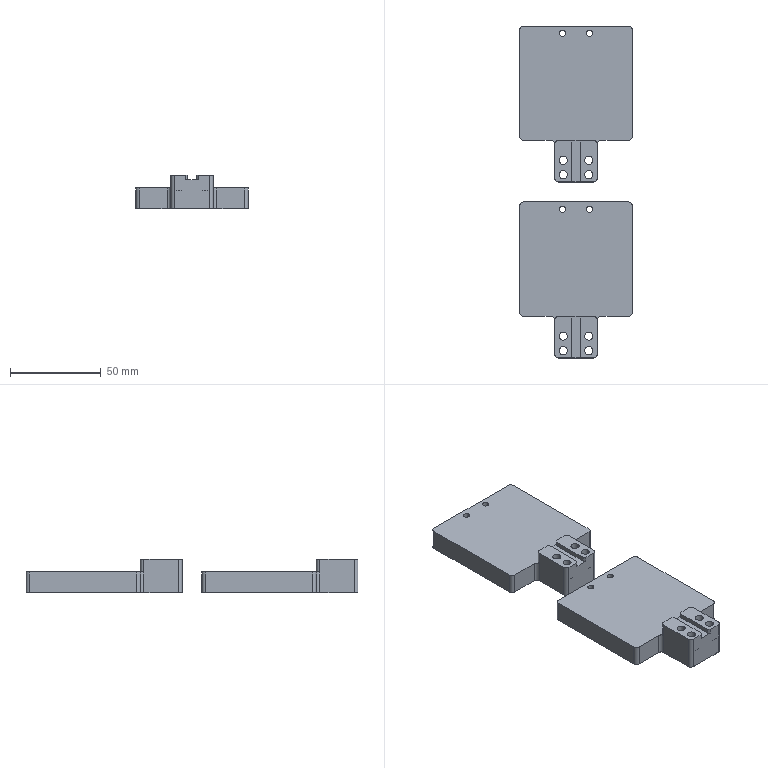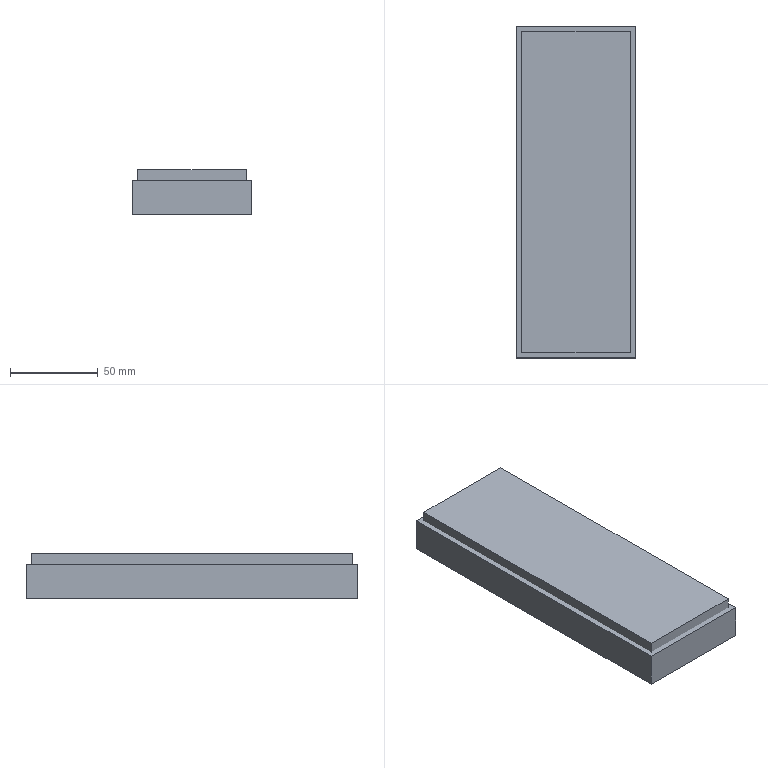CAM job | NX | 3-axis milling, drilling | part box 62 x 183 x 18.5 mm | stock box 68 x 189 x 25.5 mm
Tools:
number,name,description,diameter,corner_radius,flute_length,length,flutes
19,D80,Milling Tool-5 Parameters,80.0,0.0,50.0,75.0,2
15,D10,Milling Tool-5 Parameters,10.0,0.0,50.0,75.0,2
14,D10JING,Milling Tool-5 Parameters,10.0,0.0,50.0,75.0,2
1,D6A45,Milling Tool-5 Parameters,6.0,0.0,50.0,75.0,2
3,3.3ZT,Drilling Tool,3.3,0.0,35.0,50.0,2
11,D4,Milling Tool-5 Parameters,4.0,0.0,50.0,75.0,2
Operations:
program,operation,operation_type,tool,method,geometry_group,spindle_rpm,surface_speed,feed_per_tooth,feed_cut,feed_plunge,cut_length_mm,path_length_mm,cut_time_min,machine_time_min
1,FLOOR_WALL,VolumeBased25DMillingOperation,D80,METHOD,A,6500.0,1633.0,0.1154,1500.0,100.0,281.0,335.0,0.1873,0.1927
1,CAVITY_MILL,CavityMilling,D10,METHOD,A,9500.0,298.0,0.1842,3500.0,1000.0,30130.667,30576.909,8.744,8.789
1,ZLEVEL_PROFILE_1,ZLevelMilling,D10JING,METHOD,A,9500.0,298.0,0.0789,1500.0,1000.0,652.714,941.091,0.4379,0.4667
1,DRILLING,Operation,D6A45,METHOD,A,9500.0,179.0,0.0132,250.0,0.0,64.0,511.748,0.256,0.3008
1,DRILLING_COPY_COPY,Operation,3.3ZT,METHOD,A,2000.0,21.0,0.0375,150.0,0.0,138.331,578.124,0.9222,0.9662
1,DRILLING_COPY_COPY_COPY,Operation,3.3ZT,METHOD,A,2000.0,21.0,0.0375,150.0,0.0,179.931,593.116,1.2,1.241
1,HOLE_MILLING,CylinderMilling,D4,METHOD,A,9500.0,119.0,0.0789,1500.0,100.0,2721.362,3428.86,1.814,1.885
1,ZLEVEL_PROFILE_COPY,ZLevelMilling,D4,METHOD,A,9500.0,119.0,0.0789,1500.0,1000.0,1600.203,3019.036,1.137,1.278
1,PLANAR_MILL_COPY,PlanarMilling,D6A45,METHOD,A,9500.0,179.0,0.0658,1250.0,100.0,863.906,2253.205,0.6911,0.8301
2,FLOOR_WALL_COPY,VolumeBased25DMillingOperation,D80,METHOD,B,6500.0,1633.0,0.1154,1500.0,100.0,1925.0,3875.002,1.283,1.478
2,FLOOR_WALL_1,VolumeBased25DMillingOperation,D10,METHOD,B,9500.0,298.0,0.1842,3500.0,1000.0,12788.363,13408.033,3.749,3.811
2,FLOOR_WALL_1_COPY,VolumeBased25DMillingOperation,D10JING,METHOD,B,9500.0,298.0,0.0789,1500.0,1000.0,2120.855,2580.768,1.439,1.485
2,FLOOR_WALL_1_COPY_1,VolumeBased25DMillingOperation,D4,METHOD,B,9500.0,119.0,0.1053,2000.0,1000.0,893.37,1132.296,0.4672,0.4911
2,FLOOR_WALL_1_COPY_COPY,VolumeBased25DMillingOperation,D4,METHOD,B,9500.0,298.0,0.0789,1500.0,1000.0,297.238,527.674,0.2199,0.2429
2,PLANAR_MILL_COPY_COPY,PlanarMilling,D6A45,METHOD,B,9500.0,179.0,0.0658,1250.0,100.0,397.657,1286.444,0.3181,0.407
2,PLANAR_MILL_COPY_COPY_COPY,PlanarMilling,D6A45,METHOD,B,9500.0,179.0,0.0658,1250.0,100.0,507.657,1207.736,0.4061,0.4761
2,刀补4,VolumeBased25DMillingOperation,D4,METHOD,B,9500.0,298.0,0.0789,1500.0,1000.0,111.304,332.305,0.0769,0.099